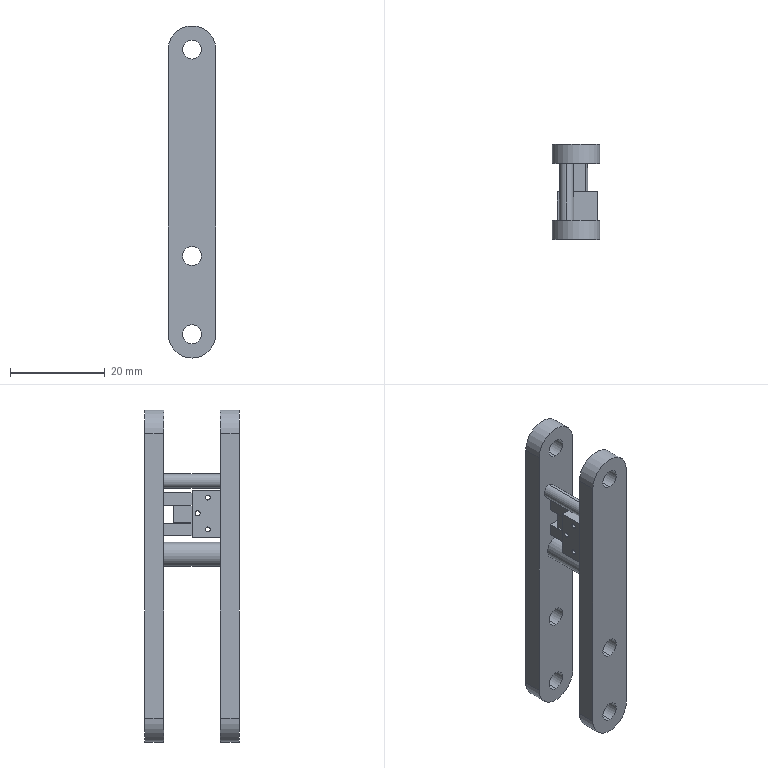Part | SolidWorks | features ICE 9, Extrusion 1 | 1 solid | 54 faces | box 10 x 20 x 70 mm | volume 6098 mm3 | cylinder 28 | plane 26 | commonest cylinder face diameters 4 x12 1.047 x6 10 x6 3 x2 5 x2